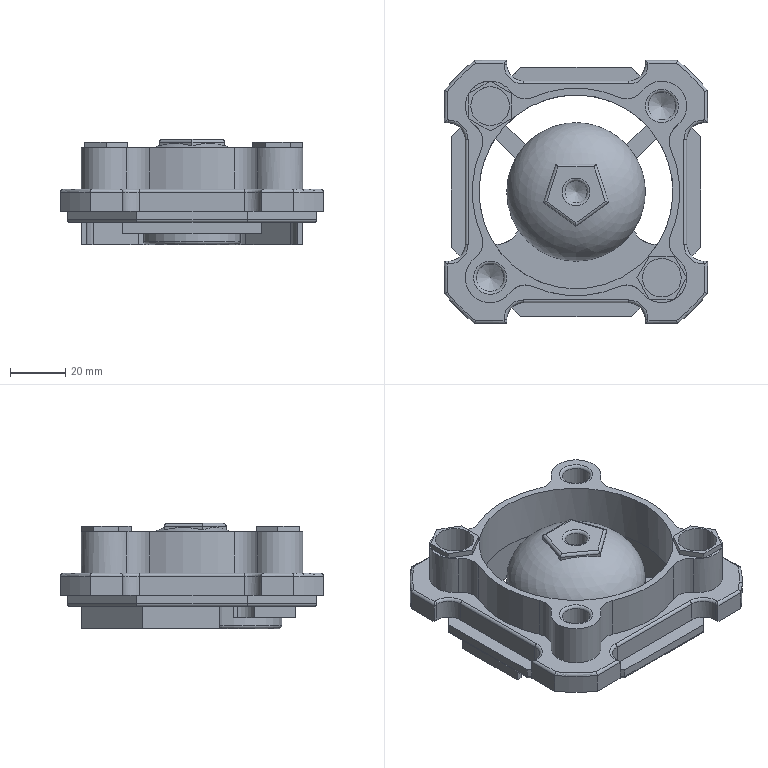NC program | NX | posted with a generic post | part box 95 x 95 x 38 mm
Lines 1 to 1357 of 59038:
N10 G17 G21 G94 G90
(FACE_MILLING , TOOL : D20)
N12 T00 M6
N14 G54
N16 G17 G0 G90 X66.539 Y-44.722 S3000 M3
N18 G43 Z10. H0
N20 Z0.2
N22 G94 G1 Z0. F2500.
N24 X53.851
N26 X-53.851
N28 G2 X-55.417 Y-42.767 R70.
N30 G1 X-57.5 Y-40.067
N32 Y-31.944
N34 X57.5
N36 Y-19.167
N38 X-57.5
N40 Y-15.
N42 X-55. Y-6.389
N44 X55.
N46 Y6.389
N48 X-55.
N50 X-57.5 Y15.
N52 Y19.167
N54 X57.5
N56 Y31.944
N58 X-57.5
N60 Y40.067
N62 X-55.417 Y42.767
N64 G2 X-53.851 Y44.722 R70.
N66 G1 X53.851
N68 X66.539
N70 Z0.2
N72 G0 Z10.
(CAVITY_MILL_COPY , TOOL : D20)
N74 X62.2 Y13.289
N76 Z-0.3
N78 G1 Z-0.5
N80 X48.2
N82 Y-47.5
N84 G2 X47.5 Y-48.2 R0.7
N86 G1 X-47.5
N88 G2 X-48.2 Y-47.5 R0.7
N90 G1 Y47.5
N92 G2 X-47.5 Y48.2 R0.7
N94 G1 X47.5
N96 G2 X48.2 Y47.5 R0.7
N98 G1 Y13.289
N100 X35.2
N102 Y-35.2
N104 X7.666
N106 Y-22.2
N108 X19.003 Y-13.963
N110 G3 X22.2 Y-10.577 R12.602
N112 G1 Y-22.2
N114 X7.666
N116 Y-35.2
N118 X-35.2
N120 Y-10.577
N122 X-22.2
N124 G3 X-19.003 Y-13.963 R12.602
N126 G1 X-7.666 Y-22.2
N128 X-22.2
N130 Y-10.577
N132 X-35.2
N134 Y35.2
N136 X-9.742
N138 Y22.2
N140 G3 X-19.152 Y13.758 R12.602
N142 G1 X-22.2 Y4.377
N144 Y22.2
N146 X-9.742
N148 X-0.007 Y24.968
N150 X-9.742 Y22.2
N152 Y35.2
N154 X35.2
N156 Y13.289
N158 X22.2
N160 Y4.377
N162 X19.152 Y13.758
N164 G3 X9.728 Y22.2 R12.625
N166 G1 X9.197 Y19.655
N168 G2 X16.679 Y12.955 R10.025
N170 G1 X21.108 Y-0.677
N172 G2 X17.475 Y-11.859 R10.002
N174 G1 X5.879 Y-20.284
N176 G2 X-5.879 Y-20.284 R10.002
N178 G1 X-17.475 Y-11.859
N180 G2 X-21.108 Y-0.677 R10.002
N182 G1 X-16.679 Y12.955
N184 G2 X-7.167 Y19.866 R10.002
N186 G1 X7.167
N188 G2 X9.197 Y19.655 R10.025
N190 G1 X9.728 Y22.2
N192 X22.2
N194 Y13.289
N196 X32.2
N198 Z-0.3
N200 G0 Z0.3
N202 X62.2 Y13.505
N204 Z-0.8
N206 G1 Z-1.
N208 X48.2
N210 Y-47.5
N212 G2 X47.5 Y-48.2 R0.7
N214 G1 X-47.5
N216 G2 X-48.2 Y-47.5 R0.7
N218 G1 Y47.5
N220 G2 X-47.5 Y48.2 R0.7
N222 G1 X47.5
N224 G2 X48.2 Y47.5 R0.7
N226 G1 Y13.505
N228 X35.2
N230 Y-35.2
N232 X7.893
N234 Y-22.2
N236 X16.314 Y-16.082
N238 X16.711 Y-15.794
N240 X19.162 Y-14.013
N242 G3 X22.2 Y-10.866 R12.608
N244 G1 Y-22.2
N246 X7.893
N248 Y-35.2
N250 X-35.2
N252 Y-10.867
N254 X-22.2
N256 G3 X-19.613 Y-13.67 R12.602
N258 G1 X-16.711 Y-15.794
N260 X-8.648 Y-21.652
N262 X-7.893 Y-22.2
N264 X-22.2
N266 Y-10.867
N268 X-35.2
N270 Y35.2
N272 X-10.415
N274 Y22.2
N276 G3 X-19.249 Y13.893 R12.6
N278 G1 X-22.2 Y4.81
N280 Y22.2
N282 X-10.415
N284 X-0.001 Y24.066
N286 X-10.415 Y22.2
N288 Y35.2
N290 X35.2
N292 Y13.505
N294 X22.2
N296 Y4.81
N298 X19.249 Y13.893
N300 G3 X10.413 Y22.2 R12.602
N302 G1 X9.763 Y19.682
N304 G2 X16.776 Y13.09 R10.002
N306 G1 X21.207 Y-0.547
N308 G2 X17.633 Y-11.91 R10.008
N310 G1 X15.183 Y-13.69
N312 X14.786 Y-13.979
N314 X5.878 Y-20.451
N316 G2 X-5.878 Y-20.451 R10.002
N318 G1 X-7.119 Y-19.549
N320 X-15.183 Y-13.69
N322 X-17.633 Y-11.91
N324 X-17.991 Y-11.637
N326 G2 X-21.205 Y-0.548 R10.002
N328 G1 X-20.851 Y0.549
N330 X-16.776 Y13.09
N332 G2 X-7.265 Y20. R10.
N334 G1 X4.929
N336 X7.265
N338 G2 X9.763 Y19.682 R10.002
N340 G1 X10.413 Y22.2
N342 X22.2
N344 Y13.505
N346 X32.2
N348 Z-0.8
N350 G0 Z0.3
N352 X-21.95 Y-62.2
N354 Z-1.3
N356 G1 Z-1.5
N358 Y-48.2
N360 X-47.5
N362 G2 X-48.2 Y-47.5 R0.7
N364 G1 Y18.116
N366 G2 X-49.384 Y19.672 R12.6
N368 X-49.519 Y19.884 R2.6
N370 G1 X-49.897 Y20.541
N372 X-49.989 Y20.717
N374 G2 X-51.394 Y26.5 R12.6
N376 G1 Y35.5
N378 G2 X-48.2 Y43.884 R12.6
N380 G1 Y47.5
N382 G2 X-47.5 Y48.2 R0.7
N384 G1 X-41.997
N386 X-37.3 Y50.912
N388 G2 X-31.752 Y52.578 R12.6
N390 X-31.445 Y52.595 R2.6
N392 G1 X-30.512 Y52.591
N394 G2 X-30.269 Y52.579 R2.6
N396 X-24.7 Y50.912 R12.6
N398 G1 X-20.003 Y48.2
N400 X47.5
N402 G2 X48.2 Y47.5 R0.7
N404 G1 Y-10.606
N406 X35.2
N408 X26.5
N410 G3 X21.702 Y-11.555 R12.6
N412 X23.739 Y0.074 R12.6
N414 G1 X19.249 Y13.894
N416 G3 X7.265 Y22.6 R12.6
N418 G1 X-7.265
N420 G3 X-11.487 Y21.872 R12.6
N422 X-10.606 Y26.5 R12.6
N424 G1 Y35.2
N426 X35.2
N428 Y20.394
N430 X26.2
N432 G3 X21.552 Y26.2 R21.6
N434 G1 X26.2
N436 Y20.394
N438 X35.2
N440 Y-10.606
N442 X48.2
N444 Y-20.003
N446 X50.912 Y-24.7
N448 G2 X52.577 Y-30.235 R12.6
N450 X52.594 Y-30.546 R2.6
N452 G1 X52.591 Y-31.481
N454 G2 X52.579 Y-31.721 R2.6
N456 X50.912 Y-37.3 R12.6
N458 G1 X48.2 Y-41.997
N460 Y-47.5
N462 G2 X47.5 Y-48.2 R0.7
N464 G1 X43.884
N466 G2 X35.5 Y-51.394 R12.6
N468 G1 X26.5
N470 G2 X20.749 Y-50.005 R12.6
N472 X20.529 Y-49.892 R2.6
N474 G1 X19.878 Y-49.516
N476 G2 X19.672 Y-49.384 R2.6
N478 X18.116 Y-48.2 R12.6
N480 G1 X-21.95
N482 Y-35.2
N484 X-35.2
N486 Y10.121
N488 G3 X-24.7 Y11.088 R12.6
N490 G1 X-19.102 Y14.32
N492 X-20.402 Y16.572
N494 X-26. Y13.34
N496 G2 X-36. Y13.34 R10.
N498 G1 X-43.794 Y17.84
N500 G2 X-47.25 Y21.162 R10.
N502 G1 X-47.264 Y21.178
N504 X-47.64 Y21.836
N506 G2 X-48.794 Y26.5 R10.
N508 G1 Y35.5
N510 G2 X-43.794 Y44.16 R10.
N512 G1 X-36. Y48.66
N514 G2 X-31.472 Y49.989 R10.
N516 G1 X-31.455 Y49.995
N518 X-30.522 Y49.989
N520 G2 X-26. Y48.66 R10.
N522 G1 X-18.206 Y44.16
N524 G2 X-13.206 Y35.5 R10.
N526 G1 Y26.5
N528 G2 X-18.206 Y17.84 R10.
N530 G1 X-20.402 Y16.572
N532 X-19.102 Y14.32
N534 G3 X-19.249 Y13.894 R12.6
N536 G1 X-23.739 Y0.074
N538 G3 X-19.162 Y-14.013 R12.6
N540 G1 X-7.406 Y-22.554
N542 G3 X7.406 Y-22.554 R12.6
N544 G1 X15.913 Y-16.374
N546 X14.385 Y-14.27
N548 X5.878 Y-20.451
N550 G2 X-5.878 Y-20.451 R10.
N552 G1 X-17.634 Y-11.91
N554 G2 X-21.266 Y-0.729 R10.
N556 G1 X-16.776 Y13.09
N558 G2 X-7.265 Y20. R10.
N560 G1 X7.265
N562 G2 X16.776 Y13.09 R10.
N564 G1 X21.266 Y-0.729
N566 G2 X17.634 Y-11.91 R10.
N568 G1 X14.385 Y-14.27
N570 X15.913 Y-16.374
N572 G3 X15.588 Y-16.906 R12.6
N574 G1 X11.088 Y-24.7
N576 G3 X10.121 Y-35.2 R12.6
N578 G1 X12.572 Y-34.333
N580 G2 X13.34 Y-26. R10.
N582 G1 X17.84 Y-18.206
N584 G2 X26.5 Y-13.206 R10.
N586 G1 X35.5
N588 G2 X44.16 Y-18.206 R10.
N590 G1 X48.66 Y-26.
N592 G2 X49.989 Y-30.522 R10.
N594 G1 X49.994 Y-30.537
N596 X49.989 Y-31.472
N598 G2 X48.66 Y-36. R10.
N600 G1 X44.16 Y-43.794
N602 G2 X35.5 Y-48.794 R10.
N604 G1 X26.5
N606 G2 X21.836 Y-47.64 R10.
N608 G1 X21.829
N610 X21.162 Y-47.25
N612 G2 X17.84 Y-43.794 R10.
N614 G1 X13.34 Y-36.
N616 G2 X12.572 Y-34.333 R10.
N618 G1 X10.121 Y-35.2
N620 X-21.95
N622 Y-26.2
N624 X-26.2
N626 Y-19.88
N628 G3 X-24.452 Y-21.294 R21.6
N630 G1 X-17.7 Y-26.2
N632 X-21.95
N634 Y-62.2
N636 Z-1.3
N638 G0 Z-0.7
N640 X-23.145
N642 Z-1.8
N644 G1 Z-2.
N646 Y-48.2
N648 X-47.5
N650 G2 X-48.2 Y-47.5 R0.7
N652 G1 Y18.116
N654 G2 X-49.384 Y19.672 R12.6
N656 X-49.519 Y19.884 R2.6
N658 G1 X-49.897 Y20.541
N660 X-49.989 Y20.717
N662 G2 X-51.394 Y26.5 R12.6
N664 G1 Y35.5
N666 G2 X-48.2 Y43.884 R12.6
N668 G1 Y47.5
N670 G2 X-47.5 Y48.2 R0.7
N672 G1 X-41.997
N674 X-37.3 Y50.912
N676 G2 X-31.752 Y52.578 R12.6
N678 X-31.445 Y52.595 R2.6
N680 G1 X-30.512 Y52.591
N682 G2 X-30.269 Y52.579 R2.6
N684 X-24.7 Y50.912 R12.6
N686 G1 X-20.003 Y48.2
N688 X47.5
N690 G2 X48.2 Y47.5 R0.7
N692 G1 Y-10.606
N694 X35.2
N696 X26.5
N698 G3 X21.702 Y-11.555 R12.6
N700 X24.011 Y-0.892 R12.6
N702 X18.909 Y14.814 R24.189
N704 X8.237 Y22.562 R12.6
N706 X-8.237 Y22.562 R24.086
N708 X-11.487 Y21.872 R12.6
N710 X-10.606 Y26.5 R12.6
N712 G1 Y35.2
N714 X35.2
N716 Y20.394
N718 X26.2
N720 G3 X21.552 Y26.2 R21.6
N722 G1 X26.2
N724 Y20.394
N726 X35.2
N728 Y-10.606
N730 X48.2
N732 Y-20.003
N734 X50.912 Y-24.7
N736 G2 X52.577 Y-30.235 R12.6
N738 X52.594 Y-30.546 R2.6
N740 G1 X52.591 Y-31.481
N742 G2 X52.579 Y-31.721 R2.6
N744 X50.912 Y-37.3 R12.6
N746 G1 X48.2 Y-41.997
N748 Y-47.5
N750 G2 X47.5 Y-48.2 R0.7
N752 G1 X43.884
N754 G2 X35.5 Y-51.394 R12.6
N756 G1 X26.5
N758 G2 X20.749 Y-50.005 R12.6
N760 X20.529 Y-49.892 R2.6
N762 G1 X19.878 Y-49.516
N764 G2 X19.672 Y-49.384 R2.6
N766 X18.116 Y-48.2 R12.6
N768 G1 X-23.145
N770 Y-35.2
N772 X-35.2
N774 Y10.121
N776 G3 X-24.7 Y11.088 R12.6
N778 G1 X-19.419 Y14.137
N780 X-20.719 Y16.389
N782 X-26. Y13.34
N784 G2 X-36. Y13.34 R10.
N786 G1 X-43.794 Y17.84
N788 G2 X-47.25 Y21.162 R10.
N790 G1 X-47.264 Y21.178
N792 X-47.64 Y21.836
N794 G2 X-48.794 Y26.5 R10.
N796 G1 Y35.5
N798 G2 X-43.794 Y44.16 R10.
N800 G1 X-36. Y48.66
N802 G2 X-31.472 Y49.989 R10.
N804 G1 X-31.455 Y49.995
N806 X-30.522 Y49.989
N808 G2 X-26. Y48.66 R10.
N810 G1 X-18.206 Y44.16
N812 G2 X-13.206 Y35.5 R10.
N814 G1 Y26.5
N816 G2 X-18.206 Y17.84 R10.
N818 G1 X-20.719 Y16.389
N820 X-19.419 Y14.137
N822 G3 X-24.011 Y-0.892 R24.19
N824 X-19.946 Y-13.395 R12.6
N826 X-6.596 Y-23.096 R24.13
N828 X6.596 Y-23.096 R12.6
N830 X14.142 Y-19.411 R24.13
N832 G1 X12.612 Y-17.309
N834 G2 X5.526 Y-20.695 R21.53
N836 X-5.526 Y-20.695 R10.
N838 X-17.991 Y-11.637 R21.53
N840 X-21.397 Y-1.165 R10.
N842 X-16.633 Y13.501 R21.59
N844 X-7.691 Y19.991 R10.
N846 X7.691 Y19.991 R21.486
N848 X16.633 Y13.501 R10.
N850 X21.397 Y-1.165 R21.589
N852 X17.991 Y-11.637 R10.
N854 X12.612 Y-17.309 R21.53
N856 G1 X14.142 Y-19.411
N858 X11.088 Y-24.7
N860 G3 X10.121 Y-35.2 R12.6
N862 G1 X12.572 Y-34.333
N864 G2 X13.34 Y-26. R10.
N866 G1 X17.84 Y-18.206
N868 G2 X26.5 Y-13.206 R10.
N870 G1 X35.5
N872 G2 X44.16 Y-18.206 R10.
N874 G1 X48.66 Y-26.
N876 G2 X49.989 Y-30.522 R10.
N878 G1 X49.994 Y-30.537
N880 X49.989 Y-31.472
N882 G2 X48.66 Y-36. R10.
N884 G1 X44.16 Y-43.794
N886 G2 X35.5 Y-48.794 R10.
N888 G1 X26.5
N890 G2 X21.836 Y-47.64 R10.
N892 G1 X21.829
N894 X21.162 Y-47.25
N896 G2 X17.84 Y-43.794 R10.
N898 G1 X13.34 Y-36.
N900 G2 X12.572 Y-34.333 R10.
N902 G1 X10.121 Y-35.2
N904 X-23.145
N906 Y-26.2
N908 X-26.2
N910 Y-20.102
N912 G3 X-20.091 Y-26.2 R33.13
N914 G1 X-23.145
N916 Y-62.2
N918 Z-1.8
N920 G0 Z-1.2
N922 X-24.158
N924 Z-2.3
N926 G1 Z-2.5
N928 Y-48.2
N930 X-47.5
N932 G2 X-48.2 Y-47.5 R0.7
N934 G1 Y18.116
N936 G2 X-49.384 Y19.672 R12.6
N938 X-49.519 Y19.884 R2.6
N940 G1 X-49.897 Y20.541
N942 X-49.989 Y20.717
N944 G2 X-51.394 Y26.5 R12.6
N946 G1 Y35.5
N948 G2 X-48.2 Y43.884 R12.6
N950 G1 Y47.5
N952 G2 X-47.5 Y48.2 R0.7
N954 G1 X-41.997
N956 X-37.3 Y50.912
N958 G2 X-31.752 Y52.578 R12.6
N960 X-31.445 Y52.595 R2.6
N962 G1 X-30.512 Y52.591
N964 G2 X-30.269 Y52.579 R2.6
N966 X-24.7 Y50.912 R12.6
N968 G1 X-20.003 Y48.2
N970 X47.5
N972 G2 X48.2 Y47.5 R0.7
N974 G1 Y-10.606
N976 X35.2
N978 X26.5
N980 G3 X22.67 Y-11.202 R12.6
N982 X-11.202 Y22.67 R25.286
N984 X-10.606 Y26.5 R12.6
N986 G1 Y35.2
N988 X35.2
N990 Y22.116
N992 X26.2
N994 G3 X22.116 Y26.2 R34.286
N996 G1 X26.2
N998 Y22.116
N1000 X35.2
N1002 Y-10.606
N1004 X48.2
N1006 Y-20.003
N1008 X50.912 Y-24.7
N1010 G2 X52.577 Y-30.235 R12.6
N1012 X52.594 Y-30.546 R2.6
N1014 G1 X52.591 Y-31.481
N1016 G2 X52.579 Y-31.721 R2.6
N1018 X50.912 Y-37.3 R12.6
N1020 G1 X48.2 Y-41.997
N1022 Y-47.5
N1024 G2 X47.5 Y-48.2 R0.7
N1026 G1 X43.884
N1028 G2 X35.5 Y-51.394 R12.6
N1030 G1 X26.5
N1032 G2 X20.749 Y-50.005 R12.6
N1034 X20.529 Y-49.892 R2.6
N1036 G1 X19.878 Y-49.516
N1038 G2 X19.672 Y-49.384 R2.6
N1040 X18.116 Y-48.2 R12.6
N1042 G1 X-24.158
N1044 Y-35.2
N1046 X-35.2
N1048 Y10.121
N1050 G3 X-24.7 Y11.088 R12.6
N1052 G1 X-21.844 Y12.737
N1054 X-23.144 Y14.988
N1056 X-26. Y13.34
N1058 G2 X-36. Y13.34 R10.
N1060 G1 X-43.794 Y17.84
N1062 G2 X-47.25 Y21.162 R10.
N1064 G1 X-47.264 Y21.178
N1066 X-47.64 Y21.836
N1068 G2 X-48.794 Y26.5 R10.
N1070 G1 Y35.5
N1072 G2 X-43.794 Y44.16 R10.
N1074 G1 X-36. Y48.66
N1076 G2 X-31.472 Y49.989 R10.
N1078 G1 X-31.455 Y49.995
N1080 X-30.522 Y49.989
N1082 G2 X-26. Y48.66 R10.
N1084 G1 X-18.206 Y44.16
N1086 G2 X-13.206 Y35.5 R10.
N1088 G1 Y26.5
N1090 G2 X-18.206 Y17.84 R10.
N1092 G1 X-23.144 Y14.988
N1094 X-21.844 Y12.737
N1096 G3 X12.737 Y-21.845 R25.286
N1098 G1 X11.427 Y-19.599
N1100 G2 X-19.598 Y-11.427 R22.686
N1102 X11.427 Y-19.599 R-22.686
N1104 G1 X12.737 Y-21.845
N1106 X11.088 Y-24.7
N1108 G3 X10.121 Y-35.2 R12.6
N1110 G1 X12.572 Y-34.333
N1112 G2 X13.34 Y-26. R10.
N1114 G1 X17.84 Y-18.206
N1116 G2 X26.5 Y-13.206 R10.
N1118 G1 X35.5
N1120 G2 X44.16 Y-18.206 R10.
N1122 G1 X48.66 Y-26.
N1124 G2 X49.989 Y-30.522 R10.
N1126 G1 X49.994 Y-30.537
N1128 X49.989 Y-31.472
N1130 G2 X48.66 Y-36. R10.
N1132 G1 X44.16 Y-43.794
N1134 G2 X35.5 Y-48.794 R10.
N1136 G1 X26.5
N1138 G2 X21.836 Y-47.64 R10.
N1140 G1 X21.829
N1142 X21.162 Y-47.25
N1144 G2 X17.84 Y-43.794 R10.
N1146 G1 X13.34 Y-36.
N1148 G2 X12.572 Y-34.333 R10.
N1150 G1 X10.121 Y-35.2
N1152 X-24.158
N1154 Y-26.2
N1156 X-26.2
N1158 Y-22.116
N1160 G3 X-22.116 Y-26.2 R34.286
N1162 G1 X-24.158
N1164 Y-62.2
N1166 Z-2.3
N1168 G0 Z-1.7
N1170 X-24.98
N1172 Z-2.8
N1174 G1 Z-3.
N1176 Y-48.2
N1178 X-47.5
N1180 G2 X-48.2 Y-47.5 R0.7
N1182 G1 Y18.116
N1184 G2 X-49.384 Y19.672 R12.6
N1186 X-49.519 Y19.884 R2.6
N1188 G1 X-49.897 Y20.541
N1190 X-49.989 Y20.717
N1192 G2 X-51.394 Y26.5 R12.6
N1194 G1 Y35.5
N1196 G2 X-48.2 Y43.884 R12.6
N1198 G1 Y47.5
N1200 G2 X-47.5 Y48.2 R0.7
N1202 G1 X-41.997
N1204 X-37.3 Y50.912
N1206 G2 X-31.752 Y52.578 R12.6
N1208 X-31.445 Y52.595 R2.6
N1210 G1 X-30.512 Y52.591
N1212 G2 X-30.269 Y52.579 R2.6
N1214 X-24.7 Y50.912 R12.6
N1216 G1 X-20.003 Y48.2
N1218 X47.5
N1220 G2 X48.2 Y47.5 R0.7
N1222 G1 Y-10.606
N1224 X35.2
N1226 X26.5
N1228 G3 X24.034 Y-10.849 R12.6
N1230 X-10.849 Y24.034 R26.37
N1232 X-10.606 Y26.5 R12.6
N1234 G1 Y35.2
N1236 X35.2
N1238 Y23.761
N1240 X26.2
N1242 G3 X23.761 Y26.2 R35.37
N1244 G1 X26.2
N1246 Y23.761
N1248 X35.2
N1250 Y-10.606
N1252 X48.2
N1254 Y-20.003
N1256 X50.912 Y-24.7
N1258 G2 X52.577 Y-30.235 R12.6
N1260 X52.594 Y-30.546 R2.6
N1262 G1 X52.591 Y-31.481
N1264 G2 X52.579 Y-31.721 R2.6
N1266 X50.912 Y-37.3 R12.6
N1268 G1 X48.2 Y-41.997
N1270 Y-47.5
N1272 G2 X47.5 Y-48.2 R0.7
N1274 G1 X43.884
N1276 G2 X35.5 Y-51.394 R12.6
N1278 G1 X26.5
N1280 G2 X20.749 Y-50.005 R12.6
N1282 X20.529 Y-49.892 R2.6
N1284 G1 X19.878 Y-49.516
N1286 G2 X19.672 Y-49.384 R2.6
N1288 X18.116 Y-48.2 R12.6
N1290 G1 X-24.98
N1292 Y-35.2
N1294 X-35.2
N1296 Y10.121
N1298 G3 X-24.7 Y11.088 R12.6
N1300 G1 X-23.629 Y11.707
N1302 X-24.929 Y13.958
N1304 X-26. Y13.34
N1306 G2 X-36. Y13.34 R10.
N1308 G1 X-43.794 Y17.84
N1310 G2 X-47.25 Y21.162 R10.
N1312 G1 X-47.264 Y21.178
N1314 X-47.64 Y21.836
N1316 G2 X-48.794 Y26.5 R10.
N1318 G1 Y35.5
N1320 G2 X-43.794 Y44.16 R10.
N1322 G1 X-36. Y48.66
N1324 G2 X-31.472 Y49.989 R10.
N1326 G1 X-31.455 Y49.995
N1328 X-30.522 Y49.989
N1330 G2 X-26. Y48.66 R10.
N1332 G1 X-18.206 Y44.16
N1334 G2 X-13.206 Y35.5 R10.
N1336 G1 Y26.5
N1338 G2 X-18.206 Y17.84 R10.
N1340 G1 X-24.929 Y13.958
N1342 X-23.629 Y11.707
N1344 G3 X11.707 Y-23.629 R26.37
N1346 G1 X10.552 Y-21.299
N1348 G2 X-21.299 Y-10.552 R23.77
N1350 X10.552 Y-21.299 R-23.77
N1352 G1 X11.707 Y-23.629
N1354 X11.088 Y-24.7
N1356 G3 X10.121 Y-35.2 R12.6
N1358 G1 X12.572 Y-34.333
N1360 G2 X13.34 Y-26. R10.
N1362 G1 X17.84 Y-18.206
N1364 G2 X26.5 Y-13.206 R10.
N1366 G1 X35.5
N1368 G2 X44.16 Y-18.206 R10.
N1370 G1 X48.66 Y-26.
N1372 G2 X49.989 Y-30.522 R10.
N1374 G1 X49.994 Y-30.537
N1376 X49.989 Y-31.472
N1378 G2 X48.66 Y-36. R10.
N1380 G1 X44.16 Y-43.794
N1382 G2 X35.5 Y-48.794 R10.
N1384 G1 X26.5
N1386 G2 X21.836 Y-47.64 R10.
N1388 G1 X21.829
N1390 X21.162 Y-47.25
N1392 G2 X17.84 Y-43.794 R10.
N1394 G1 X13.34 Y-36.
N1396 G2 X12.572 Y-34.333 R10.
N1398 G1 X10.121 Y-35.2
N1400 X-24.98
N1402 Y-26.2
N1404 X-26.2
N1406 Y-23.761
N1408 G3 X-23.761 Y-26.2 R35.37
N1410 G1 X-24.98
N1412 Y-62.2
N1414 Z-2.8
N1416 G0 Z10.
N1418 M5
(CAVITY_MILL , TOOL : F10)
N1420 M6
N1422 G54
N1424 G17 G0 G90 X-20.098 Y-1.557 S3000 M3
N1426 G43 Z10. H0
N1428 Z-2.8
N1430 G94 G3 X-20.098 Y-1.557 Z-3.458 I-3.685 J1.557 F2500.
N1432 X-19.782 Y0. Z-3.5 R4.
N1434 G2 X0. Y19.782 R19.782
N1436 X-19.782 Y0. R-19.782
N1438 G1 X-23.5
N1440 G3 X0. Y-23.5 R23.5
N1442 X-23.5 Y0. R-23.5
N1444 G1 X-30.
N1446 G3 X0. Y-30. R30.
N1448 X-30. Y0. R-30.
N1450 G1 X-25.
N1452 Z-3.3
N1454 G0 Z10.
N1456 X21.006 Y1.557
N1458 Z-3.3
N1460 G3 X21.006 Y1.557 Z-3.958 I3.685 J-1.557
N1462 X20.691 Y0. Z-4. R4.
N1464 G2 X0. Y-20.691 R20.691
N1466 X20.691 Y0. R-20.691
N1468 G1 X23.5
N1470 G3 X0. Y23.5 R23.5
N1472 X23.5 Y0. R-23.5
N1474 G1 X30.
N1476 G3 X0. Y30. R30.
N1478 X30. Y0. R-30.
N1480 G1 X25.
N1482 Z-3.8
N1484 G0 Z10.
N1486 X-21.822 Y-1.557
N1488 Z-3.8
N1490 G3 X-21.822 Y-1.557 Z-4.458 I-3.685 J1.557
N1492 X-21.506 Y0. Z-4.5 R4.
N1494 G2 X0. Y21.506 R21.506
N1496 X-21.506 Y0. R-21.506
N1498 G1 X-23.5
N1500 G3 X0. Y-23.5 R23.5
N1502 X-23.5 Y0. R-23.5
N1504 G1 X-30.
N1506 G3 X0. Y-30. R30.
N1508 X-30. Y0. R-30.
N1510 G1 X-25.
N1512 Z-4.3
N1514 G0 Z-3.7
N1516 X-23.9 Y-1.549
N1518 Z-4.3
N1520 G3 X-23.9 Y-1.549 Z-4.555 I-0.05 J1.549
N1522 X-23.9 Y-1.549 Z-4.81 I-0.05 J1.549
N1524 X-25.5 Y0. Z-5. R-1.55
N1526 X0. Y-25.5 R25.5
N1528 X-25.5 Y0. R-25.5
N1530 G1 X-30.
N1532 G3 X-17.125 Y24.632 R-30.
N1534 G1 X-12.714 Y18.288
N1536 G2 X18.288 Y12.714 R22.273
N1538 X-12.714 Y18.288 R-22.273
N1540 G1 X-17.125 Y24.632
N1542 G3 X-30. Y0. R30.
N1544 G1 X-25.
N1546 Z-4.8
N1548 G0 Z-4.2
N1550 X-23.149 Y-0.338
N1552 Z-4.8
N1554 G3 X-23.149 Y-0.338 Z-4.997 I-1.151 J0.338
N1556 X-23.149 Y-0.338 Z-5.195 I-1.151 J0.338
N1558 X-23.149 Y-0.338 Z-5.392 I-1.151 J0.338
N1560 X-25.5 Y0. Z-5.5 R-1.2
N1562 X0. Y-25.5 R25.5
N1564 X-25.5 Y0. R-25.5
N1566 G1 X-30.
N1568 G3 X-17.125 Y24.632 R-30.
N1570 G1 X-13.11 Y18.856
N1572 G2 X18.856 Y13.109 R22.966
N1574 X-13.11 Y18.856 R-22.966
N1576 G1 X-17.125 Y24.632
N1578 G3 X-30. Y0. R30.
N1580 G1 X-25.
N1582 Z-5.3
N1584 G0 Z-4.7
N1586 X-25.5 Y0.028
N1588 Z-5.3
N1590 G3 X-25.5 Y0.028 Z-5.44 I0.85 J-0.028
N1592 X-25.5 Y0.028 Z-5.58 I0.85 J-0.028
N1594 X-25.5 Y0.028 Z-5.72 I0.85 J-0.028
N1596 X-25.5 Y0.028 Z-5.859 I0.85 J-0.028
N1598 X-25.5 Y0.028 Z-5.999 I0.85 J-0.028
N1600 X-25.5 Y0. Z-6. R0.85
N1602 X0. Y-25.5 R25.5
N1604 X-25.5 Y0. R-25.5
N1606 G1 X-30.
N1608 G3 X-17.125 Y24.632 R-30.
N1610 G1 X-13.479 Y19.387
N1612 G2 X19.387 Y13.479 R23.612
N1614 X-13.479 Y19.387 R-23.612
N1616 G1 X-17.125 Y24.632
N1618 G3 X-30. Y0. R30.
N1620 G1 X-25.
N1622 Z-5.8
N1624 G0 Z10.
N1626 X28.51 Y-1.965
N1628 Z-5.8
N1630 G3 X28.51 Y-1.965 Z-6.228 I-1.703 J1.965
N1632 X24.208 Y0. Z-6.5 R-2.6
N1634 G2 X0. Y-24.208 R24.208
N1636 X24.208 Y0. R-24.208
N1638 G1 X30.
N1640 G3 X0. Y30. R30.
N1642 X30. Y0. R-30.
N1644 G1 X25.
N1646 Z-6.3
N1648 G0 Z10.
N1650 X-1.965 Y-29.078
N1652 Z-6.3
N1654 G3 X-1.965 Y-29.078 Z-6.728 I1.965 J1.703
N1656 X0. Y-24.775 Z-7. R-2.6
N1658 G2 X-24.775 Y0. R24.775
N1660 X0. Y-24.775 R-24.775
N1662 G1 Y-30.
N1664 G3 X30. Y0. R30.
N1666 X0. Y-30. R-30.
N1668 G1 Y-25.
N1670 Z-6.8
N1672 G0 Z10.
N1674 X25.803 Y-1.424
N1676 Z-6.8
N1678 G3 X25.803 Y-1.424 Z-7.17 I1.742 J1.424
N1680 X25.294 Y0. Z-7.5 R-2.25
N1682 G2 X0. Y-25.294 R25.294
N1684 X25.294 Y0. R-25.294
N1686 G1 X30.
N1688 G3 X0. Y30. R30.
N1690 X30. Y0. R-30.
N1692 G1 X27.5
N1694 Z-7.3
N1696 G0 Z-6.7
N1698 X27.545 Y1.896
N1700 Z-7.3
N1702 G3 X27.545 Y1.896 Z-7.613 I0.129 J-1.896
N1704 X27.545 Y1.896 Z-7.925 I0.129 J-1.896
N1706 X25.774 Y0. Z-8. R1.9
N1708 G2 X0. Y-25.774 R25.774
N1710 X25.774 Y0. R-25.774
N1712 G1 X30.
N1714 G3 X0. Y30. R30.
N1716 X30. Y0. R-30.
N1718 G1 X27.5
N1720 Z-7.8
N1722 G0 Z-7.2
N1724 X27.825 Y-1.549
N1726 Z-7.8
N1728 G3 X27.825 Y-1.549 Z-8.055 I-0.05 J1.549
N1730 X27.825 Y-1.549 Z-8.31 I-0.05 J1.549
N1732 X26.224 Y0. Z-8.5 R-1.55
N1734 G2 X0. Y-26.224 R26.224
N1736 X26.224 Y0. R-26.224
N1738 G1 X30.
N1740 G3 X0. Y30. R30.
N1742 X30. Y0. R-30.
N1744 G1 X27.5
N1746 Z-8.3
N1748 G0 Z-7.7
N1750 X28.237 Y-1.549
N1752 Z-8.3
N1754 G3 X28.237 Y-1.549 Z-8.555 I-0.05 J1.549
N1756 X28.237 Y-1.549 Z-8.81 I-0.05 J1.549
N1758 X26.637 Y0. Z-9. R-1.55
N1760 G2 X0. Y-26.637 R26.637
N1762 X26.637 Y0. R-26.637
N1764 G1 X30.
N1766 G3 X0. Y30. R30.
N1768 X30. Y0. R-30.
N1770 G1 X27.5
N1772 Z-8.8
N1774 G0 Z-3.2
N1776 X-0.338 Y-29.375
N1778 Z-8.8
N1780 G3 X-0.338 Y-29.375 Z-8.997 I0.338 J1.151
N1782 X-0.338 Y-29.375 Z-9.195 I0.338 J1.151
N1784 X-0.338 Y-29.375 Z-9.392 I0.338 J1.151
N1786 X0. Y-27.023 Z-9.5 R-1.2
N1788 G2 X-27.023 Y0. R27.023
N1790 X0. Y-27.023 R-27.023
N1792 G1 Y-30.
N1794 G3 X30. Y0. R30.
N1796 X0. Y-30. R-30.
N1798 G1 Y-27.5
N1800 Z-9.3
N1802 G0 Z-8.7
N1804 X-0.338 Y-29.732
N1806 Z-9.3
N1808 G3 X-0.338 Y-29.732 Z-9.497 I0.338 J1.151
N1810 X-0.338 Y-29.732 Z-9.695 I0.338 J1.151
N1812 X-0.338 Y-29.732 Z-9.892 I0.338 J1.151
N1814 X0. Y-27.381 Z-10. R-1.2
N1816 G2 X-27.381 Y0. R27.381
N1818 X0. Y-27.381 R-27.381
N1820 G1 Y-30.
N1822 G3 X30. Y0. R30.
N1824 X0. Y-30. R-30.
N1826 G1 Y-27.5
N1828 Z-9.8
N1830 G0 Z-9.2
N1832 X0.028 Y-27.713
N1834 Z-9.8
N1836 G3 X0.028 Y-27.713 Z-9.94 I-0.028 J-0.85
N1838 X0.028 Y-27.713 Z-10.08 I-0.028 J-0.85
N1840 X0.028 Y-27.713 Z-10.22 I-0.028 J-0.85
N1842 X0.028 Y-27.713 Z-10.359 I-0.028 J-0.85
N1844 X0.028 Y-27.713 Z-10.499 I-0.028 J-0.85
N1846 X0. Y-27.712 Z-10.5 R0.85
N1848 G2 X-27.712 Y0. R27.712
N1850 X0. Y-27.712 R-27.712
N1852 G1 Y-30.
N1854 G3 X30. Y0. R30.
N1856 X0. Y-30. R-30.
N1858 G1 Z-10.3
N1860 G0 Z10.
N1862 X-0.028 Y28.017
N1864 Z-10.3
N1866 G3 X-0.028 Y28.017 Z-10.44 I0.028 J0.85
N1868 X-0.028 Y28.017 Z-10.58 I0.028 J0.85
N1870 X-0.028 Y28.017 Z-10.72 I0.028 J0.85
N1872 X-0.028 Y28.017 Z-10.859 I0.028 J0.85
N1874 X-0.028 Y28.017 Z-10.999 I0.028 J0.85
N1876 X0. Y28.017 Z-11. R0.85
N1878 G2 X28.017 Y0. R28.017
N1880 X0. Y28.017 R-28.017
N1882 G1 Y30.
N1884 G3 X-30. Y0. R30.
N1886 X0. Y30. R-30.
N1888 G1 Z-10.8
N1890 G0 Z-3.2
N1892 X-28.299 Y-0.032
N1894 Z-10.8
N1896 G3 X-28.299 Y-0.032 Z-10.94 I-0.85 J0.028
N1898 X-28.299 Y-0.032 Z-11.08 I-0.85 J0.028
N1900 X-28.299 Y-0.032 Z-11.22 I-0.85 J0.028
N1902 X-28.299 Y-0.032 Z-11.359 I-0.85 J0.028
N1904 X-28.299 Y-0.032 Z-11.499 I-0.85 J0.028
N1906 X-28.298 Y-0.003 Z-11.5 R0.85
N1908 G2 X-26.456 Y10.038 R28.287
N1910 X24.708 Y13.8 R28.3
N1912 X24.708 Y-13.8 R28.356
N1914 X-10.038 Y-26.456 R28.301
N1916 X-28.034 Y-3.861 R28.298
N1918 X-28.298 Y-0.003 R28.287
N1920 G1 X-30.
N1922 G3 X0.003 Y-30. R30.
N1924 X-30. Y-0.003 R-30.
N1926 G1 Z-11.3
N1928 G0 Z10.
N1930 X29.558 Y-0.028
N1932 Z-11.3
N1934 G3 X29.558 Y-0.028 Z-11.382 I-0.499 J0.028
N1936 X29.558 Y-0.028 Z-11.465 I-0.499 J0.028
N1938 X29.558 Y-0.028 Z-11.547 I-0.499 J0.028
N1940 X29.558 Y-0.028 Z-11.629 I-0.499 J0.028
N1942 X29.558 Y-0.028 Z-11.711 I-0.499 J0.028
N1944 X29.558 Y-0.028 Z-11.794 I-0.499 J0.028
N1946 X29.558 Y-0.028 Z-11.876 I-0.499 J0.028
N1948 X29.558 Y-0.028 Z-11.958 I-0.499 J0.028
N1950 X28.559 Y0. Z-12. R-0.5
N1952 G2 X0. Y-28.559 R28.559
N1954 X28.559 Y0. R-28.559
N1956 G1 X30.
N1958 G3 X0. Y30. R30.
N1960 X30. Y0. R-30.
N1962 G1 Z-11.8
N1964 G0 Z10.
N1966 X-29.793 Y0.028
N1968 Z-11.8
N1970 G3 X-29.793 Y0.028 Z-11.882 I0.499 J-0.028
N1972 X-29.793 Y0.028 Z-11.965 I0.499 J-0.028
N1974 X-29.793 Y0.028 Z-12.047 I0.499 J-0.028
N1976 X-29.793 Y0.028 Z-12.129 I0.499 J-0.028
N1978 X-29.793 Y0.028 Z-12.211 I0.499 J-0.028
N1980 X-29.793 Y0.028 Z-12.294 I0.499 J-0.028
N1982 X-29.793 Y0.028 Z-12.376 I0.499 J-0.028
N1984 X-29.793 Y0.028 Z-12.458 I0.499 J-0.028
N1986 X-28.793 Y0. Z-12.5 R-0.5
N1988 G2 X0. Y28.793 R28.793
N1990 X-28.793 Y0. R-28.793
N1992 G1 X-30.
N1994 G3 X0. Y-30. R30.
N1996 X-30. Y0. R-30.
N1998 G1 Z-12.3
N2000 G0 Z10.
N2002 X23.105 Y-17.533
N2004 Z-12.3
N2006 G2 X0. Y-29.004 Z-13. R29.004
N2008 X-29.004 Y0. R29.004
N2010 X0. Y-29.004 R-29.004
N2012 G1 Y-30.
N2014 G3 X30. Y0. R30.
N2016 X0. Y-30. R-30.
N2018 G1 Z-12.8
N2020 G0 Z-8.2
N2022 X23.15 Y-17.786
N2024 Z-12.8
N2026 G2 X0. Y-29.193 Z-13.5 R29.193
N2028 X-29.193 Y0. R29.193
N2030 X0. Y-29.193 R-29.193
N2032 G1 Y-30.
N2034 G3 X30. Y0. R30.
N2036 X0. Y-30. R-30.
N2038 G1 Z-13.3
N2040 G0 Z10.
N2042 X18.008 Y23.189
N2044 Z-13.3
N2046 G2 X29.36 Y0. Z-14. R29.36
N2048 X0. Y-29.36 R29.36
N2050 X29.36 Y0. R-29.36
N2052 G1 X30.
N2054 G3 X0. Y30. R30.
N2056 X30. Y0. R-30.
N2058 G1 Z-13.8
N2060 G0 Z-10.7
N2062 X23.223 Y-18.207
N2064 Z-13.8
N2066 G2 X0. Y-29.51 Z-14.5 R29.51
N2068 X-29.51 Y0. R29.51
N2070 X0. Y-29.51 R-29.51
N2072 G1 Y-30.
N2074 G3 X30. Y0. R30.
N2076 X0. Y-30. R-30.
N2078 G1 Z-14.3
N2080 G0 Z10.
N2082 X18.377 Y23.252
N2084 Z-14.3
N2086 G2 X29.637 Y0. Z-15. R29.637
N2088 X0. Y-29.637 R29.637
N2090 X29.637 Y0. R-29.637
N2092 G1 X30.
N2094 G3 X0. Y30. R30.
N2096 X30. Y0. R-30.
N2098 G1 Z-14.8
N2100 G0 Z-10.7
N2102 X23.275 Y-18.521
N2104 Z-14.8
N2106 G2 X-0.001 Y-29.746 Z-15.5 R29.745
N2108 X-29.745 Y-0.001 R29.745
N2110 X-0.001 Y-29.746 R-29.745
N2112 G1 Y-30.
N2114 G3 X30. Y-0.001 R30.
N2116 X-0.001 Y-30. R-30.
N2118 G1 Z-15.3
N2120 G0 Z-10.7
N2122 X-18.645 Y-23.296
N2124 Z-15.3
N2126 G2 X-29.84 Y0.001 Z-16. R29.839
N2128 X-0.001 Y29.84 R29.839
N2130 X-29.84 Y0.001 R-29.839
N2132 G1 X-30.
N2134 G3 X-0.001 Y-30. R30.
N2136 X-30. Y0.001 R-30.
N2138 G1 Z-15.8
N2140 G0 Z10.
N2142 X18.735 Y23.311
N2144 Z-15.8
N2146 G2 X29.907 Y-0.001 Z-16.5 R29.906
N2148 X0.001 Y-29.907 R29.906
N2150 X29.907 Y-0.001 R-29.906
N2152 G1 X30.
N2154 G3 X0.001 Y30. R30.
N2156 X30. Y-0.001 R-30.
N2158 G1 Z-16.3
N2160 G0 Z-10.2
N2162 X21.211 Y-21.175
N2164 Z-16.3
N2166 G1 X21.388 Y-21.009 Z-16.306
N2168 X22.284 Y-20.011 Z-16.341
N2170 X21.388 Y-21.009 Z-16.377
N2172 X19.519 Y-22.756 Z-16.444
N2174 X17.508 Y-24.338 Z-16.511
N2176 X15.369 Y-25.742 Z-16.578
N2178 X13.008 Y-27.012 Z-16.648
N2180 X10.217 Y-28.187 Z-16.727
N2182 X7.323 Y-29.073 Z-16.806
N2184 X4.353 Y-29.664 Z-16.886
N2186 X1.34 Y-29.952 Z-16.965
N2188 X-0.001 Z-17.
N2190 G2 X-28.569 Y-8.999 R29.951
N2192 X-29.508 Y5.095 R30.135
N2194 X-22.901 Y19.303 R29.894
N2196 X-0.001 Y-29.952 R-29.951
N2198 G1 Y-30.
N2200 G3 X30. Y-0.001 R30.
N2202 X-0.001 Y-30. R-30.
N2204 G1 Z-16.8
N2206 G0 Z-9.2
N2208 X23.328 Y-18.832
N2210 Z-16.8
N2212 G2 X0. Y-29.981 Z-17.5 R29.98
N2214 X-29.98 Y-0.002 R29.98
N2216 X0. Y-29.981 R-29.98
N2218 G1 Y-30.
N2220 G3 X30. Y0. R30.
N2222 X0. Y-30. R-30.
N2224 G1 Z-17.3
N2226 G0 Z10.
N2228 X0.785 Y30.
N2230 Z-17.3
N2232 G1 X0. Z-17.321
N2234 X0.4 Z-17.331
N2236 X0.801 Y29.989 Z-17.342
N2238 X0.4 Y30. Z-17.352
N2240 X0. Z-17.362
N2242 X1.343 Y29.999 Z-17.398
N2244 X4.711 Y29.657 Z-17.486
N2246 X8.02 Y28.937 Z-17.575
N2248 X11.227 Y27.851 Z-17.664
N2250 X14.291 Y26.411 Z-17.752
N2252 X15.443 Y25.72 Z-17.787
N2254 X14.292 Y26.411 Z-17.823
N2256 X11.847 Y27.594 Z-17.894
N2258 X9.306 Y28.552 Z-17.965
N2260 X8.012 Y28.91 Z-18.
N2262 G3 X0. Y30. R30.
N2264 G2 X15.443 Y25.72 R30.048
N2266 G3 X8.012 Y28.91 R30.
N2268 G1 Z-17.8
N2270 G0 Z10.
N2272 X-6.981 Y29.202
N2274 Z-17.3
N2276 G1 X-7.092 Y29.181 Z-17.303
N2278 X-7.878 Y28.978 Z-17.324
N2280 X-9.156 Y28.569 Z-17.359
N2282 X-7.864 Y28.979 Z-17.395
N2284 X-5.78 Y29.464 Z-17.451
N2286 X-3.668 Y29.803 Z-17.507
N2288 X-2.316 Y29.91 Z-17.542
N2290 X-3.654 Y29.807 Z-17.578
N2292 X-4.458 Y29.697 Z-17.599
N2294 X-7.092 Y29.181 Z-17.669
N2296 X-7.878 Y28.978 Z-17.69
N2298 X-9.156 Y28.569 Z-17.725
N2300 X-7.864 Y28.979 Z-17.761
N2302 X-5.78 Y29.464 Z-17.817
N2304 X-3.668 Y29.803 Z-17.873
N2306 X-2.316 Y29.91 Z-17.908
N2308 X-3.654 Y29.807 Z-17.944
N2310 X-4.458 Y29.697 Z-17.965
N2312 X-5.775 Y29.439 Z-18.
N2314 G3 X-9.156 Y28.569 R30.
N2316 G2 X-2.316 Y29.91 R30.608
N2318 G3 X-5.775 Y29.439 R30.
N2320 G1 Z-17.8
N2322 G0 Z10.
N2324 X-27.603 Y11.814
N2326 Z-17.3
N2328 G1 X-28.6 Y9.155 Z-17.374
N2330 X-29.304 Y6.565 Z-17.445
N2332 X-29.807 Y3.654 Z-17.522
N2334 X-29.91 Y2.316 Z-17.557
N2336 X-29.804 Y3.66 Z-17.592
N2338 X-29.319 Y6.478 Z-17.667
N2340 X-28.569 Y9.238 Z-17.742
N2342 X-27.563 Y11.915 Z-17.817
N2344 X-26.975 Y13.128 Z-17.852
N2346 X-27.563 Y11.921 Z-17.888
N2348 X-28.6 Y9.155 Z-17.965
N2350 X-28.952 Y7.86 Z-18.
N2352 G3 X-29.91 Y2.316 R30.
N2354 G2 X-26.975 Y13.128 R30.259
N2356 G3 X-28.952 Y7.86 R30.
N2358 G1 Z-17.8
N2360 G0 Z10.
N2362 X-29.99 Y-0.472
N2364 Z-17.3
N2366 G1 Y0.772 Z-17.333
N2368 X-30. Y0.386 Z-17.343
N2370 Y-0.386 Z-17.363
N2372 X-29.99 Y-0.772 Z-17.373
N2374 Y0.772 Z-17.413
N2376 X-30. Y0.386 Z-17.424
N2378 Y-0.386 Z-17.444
N2380 X-29.99 Y-0.772 Z-17.454
N2382 Y0.772 Z-17.494
N2384 X-30. Y0.386 Z-17.504
N2386 Y-0.386 Z-17.525
N2388 X-29.99 Y-0.772 Z-17.535
N2390 Y0.772 Z-17.575
N2392 X-30. Y0.386 Z-17.585
N2394 Y-0.386 Z-17.606
N2396 X-29.99 Y-0.772 Z-17.616
N2398 Y0.772 Z-17.656
N2400 X-30. Y0.386 Z-17.666
N2402 Y-0.386 Z-17.687
N2404 X-29.99 Y-0.772 Z-17.697
N2406 Y0.772 Z-17.737
N2408 X-30. Y0.386 Z-17.747
N2410 Y-0.386 Z-17.767
N2412 X-29.99 Y-0.772 Z-17.778
N2414 Y0.772 Z-17.818
N2416 X-30. Y0.386 Z-17.828
N2418 Y-0.386 Z-17.848
N2420 X-29.99 Y-0.772 Z-17.858
N2422 Y0.772 Z-17.899
N2424 X-30. Y0.386 Z-17.909
N2426 Y-0.386 Z-17.929
N2428 X-29.99 Y-0.772 Z-17.939
N2430 Y0.772 Z-17.98
N2432 X-30. Y0.386 Z-17.99
N2434 Y0. Z-18.
N2436 G3 X-29.99 Y-0.772 R30.
N2438 G1 Y0.772
N2440 G3 X-30. Y0. R30.
N2442 G1 Z-17.8
N2444 G0 Z10.
N2446 X-29.787 Y-3.767
N2448 Z-17.3
N2450 G1 X-29.304 Y-6.565 Z-17.374
N2452 X-28.6 Y-9.155 Z-17.445
N2454 X-27.563 Y-11.921 Z-17.522
N2456 X-26.975 Y-13.128 Z-17.557
N2458 X-27.563 Y-11.915 Z-17.592
N2460 X-28.569 Y-9.238 Z-17.667
N2462 X-29.319 Y-6.478 Z-17.742
N2464 X-29.804 Y-3.66 Z-17.817
N2466 X-29.91 Y-2.316 Z-17.852
N2468 X-29.807 Y-3.654 Z-17.888
N2470 X-29.304 Y-6.565 Z-17.965
N2472 X-28.952 Y-7.86 Z-18.
N2474 G3 X-26.975 Y-13.128 R30.
N2476 G2 X-29.91 Y-2.316 R30.25
N2478 G3 X-28.952 Y-7.86 R30.
N2480 G1 Z-17.8
N2482 G0 Z10.
N2484 X-20.27 Y-22.137
N2486 Z-17.3
N2488 G1 X-20.1 Y-22.306 Z-17.306
N2490 X-19.061 Y-23.162 Z-17.342
N2492 X-20.1 Y-22.306 Z-17.377
N2494 X-22.141 Y-20.279 Z-17.452
N2496 X-23.981 Y-18.067 Z-17.527
N2498 X-25.603 Y-15.691 Z-17.603
N2500 X-26.256 Y-14.513 Z-17.638
N2502 X-25.607 Y-15.688 Z-17.673
N2504 X-23.489 Y-18.71 Z-17.77
N2506 X-21.017 Y-21.45 Z-17.866
N2508 X-18.227 Y-23.866 Z-17.963
N2510 X-17.07 Y-24.67 Z-18.
N2512 X-17.014 Y-24.708
N2514 G2 X-26.256 Y-14.513 R30.196
N2516 G3 X-17.07 Y-24.67 R30.
N2518 G1 Z-17.8
N2520 G0 Z10.
N2522 X-12.915 Y-27.089
N2524 Z-17.3
N2526 G1 X-11.302 Y-27.822 Z-17.346
N2528 X-10.038 Y-28.271 Z-17.382
N2530 X-11.317 Y-27.812 Z-17.417
N2532 X-13.639 Y-26.747 Z-17.484
N2534 X-15.864 Y-25.493 Z-17.551
N2536 X-16.987 Y-24.727 Z-17.586
N2538 X-16.762 Y-24.88 Z-17.594
N2540 X-15.649 Y-25.63 Z-17.629
N2542 X-13.52 Y-26.814 Z-17.693
N2544 X-11.302 Y-27.822 Z-17.756
N2546 X-10.038 Y-28.271 Z-17.791
N2548 X-11.317 Y-27.812 Z-17.827
N2550 X-13.639 Y-26.747 Z-17.894
N2552 X-15.864 Y-25.493 Z-17.961
N2554 X-16.987 Y-24.727 Z-17.996
N2556 X-16.875 Y-24.804 Z-18.
N2558 X-16.762 Y-24.88
N2560 G3 X-10.038 Y-28.271 R30.
N2562 G2 X-16.987 Y-24.727 R30.766
N2564 G1 X-16.875 Y-24.804
N2566 Z-17.8
N2568 G0 Z10.
N2570 X-4.569 Y-29.676
N2572 Z-17.3
N2574 G1 X-4.458 Y-29.697 Z-17.303
N2576 X-3.654 Y-29.807 Z-17.324
N2578 X-2.316 Y-29.91 Z-17.359
N2580 X-3.668 Y-29.803 Z-17.395
N2582 X-5.78 Y-29.464 Z-17.451
N2584 X-7.864 Y-28.979 Z-17.507
N2586 X-9.156 Y-28.569 Z-17.542
N2588 X-7.878 Y-28.978 Z-17.578
N2590 X-7.092 Y-29.181 Z-17.599
N2592 X-4.458 Y-29.697 Z-17.669
N2594 X-3.654 Y-29.807 Z-17.69
N2596 X-2.316 Y-29.91 Z-17.725
N2598 X-3.668 Y-29.803 Z-17.761
N2600 X-5.78 Y-29.464 Z-17.817
N2602 X-7.864 Y-28.979 Z-17.873
N2604 X-9.156 Y-28.569 Z-17.908
N2606 X-7.878 Y-28.978 Z-17.944
N2608 X-7.092 Y-29.181 Z-17.965
N2610 X-5.775 Y-29.439 Z-18.
N2612 G3 X-2.316 Y-29.91 R30.
N2614 G2 X-9.156 Y-28.569 R30.608
N2616 G3 X-5.775 Y-29.439 R30.
N2618 G1 Z-17.8
N2620 G0 Z10.
N2622 X14.769 Y-26.123
N2624 Z-17.3
N2626 G1 X15.446 Y-25.718 Z-17.321
N2628 X15.105 Y-25.923 Z-17.331
N2630 X14.758 Y-26.119 Z-17.342
N2632 X15.105 Y-25.923 Z-17.352
N2634 X15.446 Y-25.718 Z-17.362
N2636 X14.292 Y-26.409 Z-17.398
N2638 X11.227 Y-27.847 Z-17.486
N2640 X8.021 Y-28.933 Z-17.575
N2642 X4.713 Y-29.653 Z-17.664
N2644 X1.345 Y-29.998 Z-17.752
N2646 X0. Y-30. Z-17.787
N2648 X1.342 Z-17.823
N2650 X4.048 Y-29.756 Z-17.894
N2652 X6.721 Y-29.268 Z-17.965
N2654 X8.014 Y-28.91 Z-18.
N2656 G3 X15.446 Y-25.718 R30.
N2658 G2 X0. Y-30. R30.151
N2660 G3 X8.014 Y-28.91 R30.
N2662 G1 Z-17.8
N2664 G0 Z10.
N2666 X21.236 Y-21.212
N2668 Z-17.3
N2670 G1 X21.071 Y-21.396 Z-17.306
N2672 X20.074 Y-22.294 Z-17.342
N2674 X21.071 Y-21.396 Z-17.377
N2676 X23.569 Y-18.609 Z-17.475
N2678 X25.701 Y-15.532 Z-17.573
N2680 X27.434 Y-12.214 Z-17.671
N2682 X28.74 Y-8.707 Z-17.769
N2684 X29.6 Y-5.064 Z-17.867
N2686 X30. Y-1.342 Z-17.965
N2688 Y0. Z-18.
N2690 G3 X16.215 Y25.241 R30.
N2692 G2 X16.215 Y-25.241 R30.005
N2694 G3 X30. Y0. R30.
N2696 G1 Z-17.8
N2698 G0 Z10.
N2700 M5